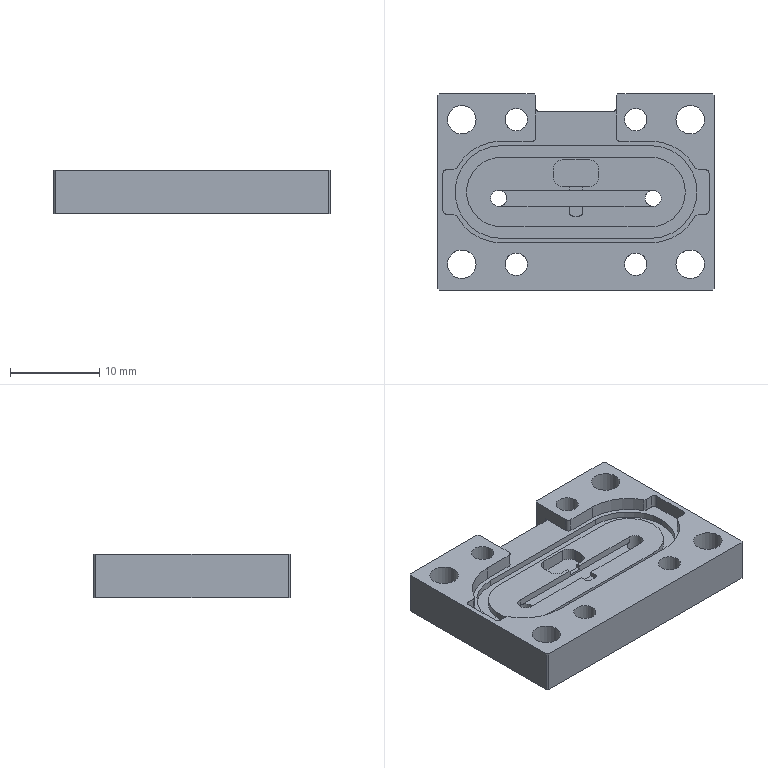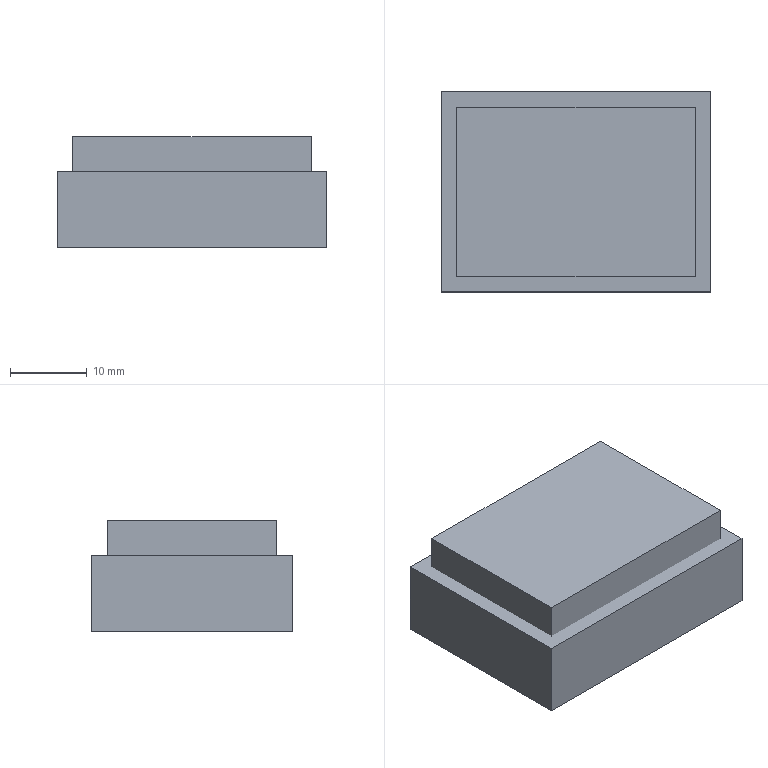CAM job | NX | 3-axis milling, drilling | part box 31 x 22 x 4.9 mm | stock box 35 x 26 x 14.4 mm
Tools:
number,name,description,diameter,corner_radius,flute_length,length,flutes
10,D0.8,Milling Tool-5 Parameters,0.8,0.0,4.0,65.0,2
13,D2.5钻头,Drilling Tool,2.5,0.0,35.0,50.0,2
8,D3.2钻头,Drilling Tool,3.2,0.0,35.0,50.0,2
14,螺纹铣刀M3,Thread Mill,2.4,0.0,2.0,50.0,3
12,D50面刀,Milling Tool-5 Parameters,50.0,0.0,30.0,100.0,2
1,D45面刀,Milling Tool-5 Parameters,50.0,0.0,30.0,100.0,2
2,6C-15L-25L,Milling Tool-5 Parameters,6.0,0.0,15.0,65.0,2
3,5J-15L-25L,Milling Tool-5 Parameters,5.0,0.0,15.0,65.0,2
16,4J-10L-25L,Milling Tool-5 Parameters,4.0,0.0,10.0,65.0,2
15,4C-10L-25L,Milling Tool-5 Parameters,4.0,0.0,10.0,65.0,2
4,1.5C-4L-15L,Milling Tool-5 Parameters,1.5,0.0,4.0,65.0,2
5,1C-4L-15L,Milling Tool-5 Parameters,1.0,0.0,4.0,65.0,2
6,1J-4L-15L,Milling Tool-5 Parameters,1.0,0.0,4.0,65.0,2
7,D5点钻,Drilling Tool,5.0,0.0,10.0,75.0,2
9,D2点钻,Drilling Tool,2.0,0.0,10.0,75.0,2
Operations:
program,operation,operation_type,tool,method,geometry_group,spindle_rpm,surface_speed,feed_per_tooth,feed_cut,feed_plunge,cut_length_mm,path_length_mm,cut_time_min,machine_time_min
A0101,FACE_MILLING,FaceMilling,D50面刀,METHOD,W1,1600.0,251.0,0.1875,600.0,100.0,182.0,339.85,0.3033,0.3191
A0102,ADAPTIVE_MILLING,CavityMilling,6C-15L-25L,METHOD,W1,4500.0,84.0,0.1667,1500.0,100.0,1190.413,1236.213,0.7936,0.7982
A0103,DRILLING,Operation,D5点钻,METHOD,W1,1200.0,18.0,0.0417,100.0,0.0,32.0,196.13,0.32,0.3364
A0104,DRILLING_1,Operation,D3.2钻头,METHOD,W1,1600.0,16.0,0.025,80.0,0.0,41.446,190.617,0.5181,0.533
A0105,DRILLING_2,Operation,D2.5钻头,METHOD,W1,3000.0,23.0,0.01,60.0,0.0,38.0,168.939,0.6333,0.6464
A0106,DRILLING_COPY,Operation,D5点钻,METHOD,W1,2000.0,31.0,0.02,80.0,0.0,18.4,153.826,0.23,0.2435
A0106,DRILLING_COPY_1,Operation,D5点钻,METHOD,W1,2000.0,31.0,0.02,80.0,0.0,17.6,128.139,0.22,0.2311
A0107,THREAD_MILLING,ThreadMilling,螺纹铣刀M3,METHOD,W1,3500.0,26.0,0.0076,80.0,100.0,246.236,1010.836,3.078,3.154
A0108,PLANAR_MILL,PlanarMilling,5J-15L-25L,METHOD,W1,3000.0,47.0,0.0667,400.0,100.0,383.518,529.718,0.9588,0.9734
A0109,FACE_MILLING_COPY,FaceMilling,D45面刀,METHOD,W1,5500.0,863.0,0.0273,300.0,100.0,91.0,127.0,0.3033,0.3069
A0110,PLANAR_MILL_1,PlanarMilling,D2点钻,METHOD,W1,3000.0,28.0,0.0667,400.0,100.0,110.273,145.273,0.2757,0.2792
A0113,DRILLING_COPY_1_COPY,Operation,D5点钻,METHOD,W1,2000.0,31.0,0.02,80.0,0.0,7.8,76.158,0.0975,0.1043
A0113,HOLE_MILLING,CylinderMilling,1.5C-4L-15L,METHOD,W1,3500.0,16.0,0.0143,100.0,100.0,125.522,227.322,1.255,1.265
B0101,FACE_MILLING_1,FaceMilling,D50面刀,METHOD,W2,1600.0,251.0,0.25,800.0,100.0,1274.0,2856.25,1.593,1.751
B0102,FACE_MILLING_2,FaceMilling,4C-10L-25L,METHOD,W2,3000.0,37.0,0.2,1200.0,100.0,1089.4,1447.488,0.9078,0.9436
B0103,PLANAR_MILL_4,PlanarMilling,1.5C-4L-15L,METHOD,W2,3500.0,16.0,0.0714,500.0,100.0,386.548,632.678,0.7731,0.7977
B0103,PLANAR_MILL_4_COPY,PlanarMilling,1.5C-4L-15L,METHOD,W2,3500.0,16.0,0.0714,500.0,100.0,1119.35,1857.455,2.239,2.312
B0103,PLANAR_MILL_3,PlanarMilling,1.5C-4L-15L,METHOD,W2,3500.0,16.0,0.0714,500.0,100.0,795.817,836.417,1.592,1.596
B0103,PLANAR_MILL_3_COPY,PlanarMilling,1.5C-4L-15L,METHOD,W2,3500.0,16.0,0.0714,500.0,100.0,1393.942,1438.092,2.788,2.792
B0104,PLANAR_MILL_2,PlanarMilling,1C-4L-15L,METHOD,W2,4000.0,12.0,0.0375,300.0,100.0,921.84,965.289,3.073,3.077
B0104,PLANAR_MILL_2_COPY,PlanarMilling,1C-4L-15L,METHOD,W2,4000.0,12.0,0.0375,300.0,100.0,637.554,680.804,2.125,2.13
B0105,FACE_MILLING_2_COPY,FaceMilling,4J-10L-25L,METHOD,W2,3000.0,37.0,0.05,300.0,100.0,138.213,175.213,0.4607,0.4644
B0105,FACE_MILLING_2_COPY_COPY,FaceMilling,4J-10L-25L,METHOD,W2,3000.0,37.0,0.05,300.0,100.0,79.924,116.924,0.2664,0.2701
B0106,PLANAR_MILL_4_COPY_1,PlanarMilling,D0.8,METHOD,W2,3500.0,8.0,0.0286,200.0,100.0,456.341,727.686,2.282,2.309
B0106,PLANAR_MILL_4_COPY_COPY,PlanarMilling,D0.8,METHOD,W2,3500.0,8.0,0.0286,200.0,100.0,1221.008,1994.106,6.105,6.182
B0106,PLANAR_MILL_2_COPY_COPY,PlanarMilling,D0.8,METHOD,W2,3500.0,8.0,0.0286,200.0,100.0,121.0,542.487,0.605,0.6471
B0107,PLANAR_MILL_3_COPY_1,PlanarMilling,1J-4L-15L,METHOD,W2,3000.0,9.0,0.0333,200.0,100.0,68.96,107.46,0.3448,0.3486
B0107,PLANAR_MILL_3_COPY_COPY,PlanarMilling,1J-4L-15L,METHOD,W2,3000.0,9.0,0.0333,200.0,100.0,28.062,73.662,0.1403,0.1449
B0107,PLANAR_MILL_2_COPY_1,PlanarMilling,1J-4L-15L,METHOD,W2,3000.0,9.0,0.0333,200.0,100.0,254.341,342.359,1.272,1.28
B0108,FACE_MILLING_1_COPY,FaceMilling,D45面刀,METHOD,W2,5500.0,251.0,0.25,300.0,100.0,91.0,127.0,0.3033,0.3069
B0109,DRILLING_3,Operation,D5点钻,METHOD,W2,2000.0,31.0,0.05,200.0,0.0,18.4,153.826,0.092,0.1055
B0109,DRILLING_3_COPY,Operation,D5点钻,METHOD,W2,2000.0,31.0,0.05,200.0,0.0,17.6,128.139,0.088,0.0991
B0110,PLANAR_MILL_5,PlanarMilling,D2点钻,METHOD,W2,3000.0,18.0,0.0833,500.0,100.0,180.237,216.837,0.3605,0.3641
B0110,PLANAR_MILL_6,PlanarMilling,D2点钻,METHOD,W2,3000.0,18.0,0.0833,500.0,100.0,54.383,138.242,0.1088,0.1172
B0110,PLANAR_MILL_6_COPY,PlanarMilling,D2点钻,METHOD,W2,3000.0,18.0,0.0833,500.0,100.0,128.705,168.705,0.2574,0.2614
B0110,PLANAR_MILL_2_COPY_COPY_1,PlanarMilling,D2点钻,METHOD,W2,3000.0,18.0,0.0833,500.0,100.0,13.5,53.5,0.027,0.031